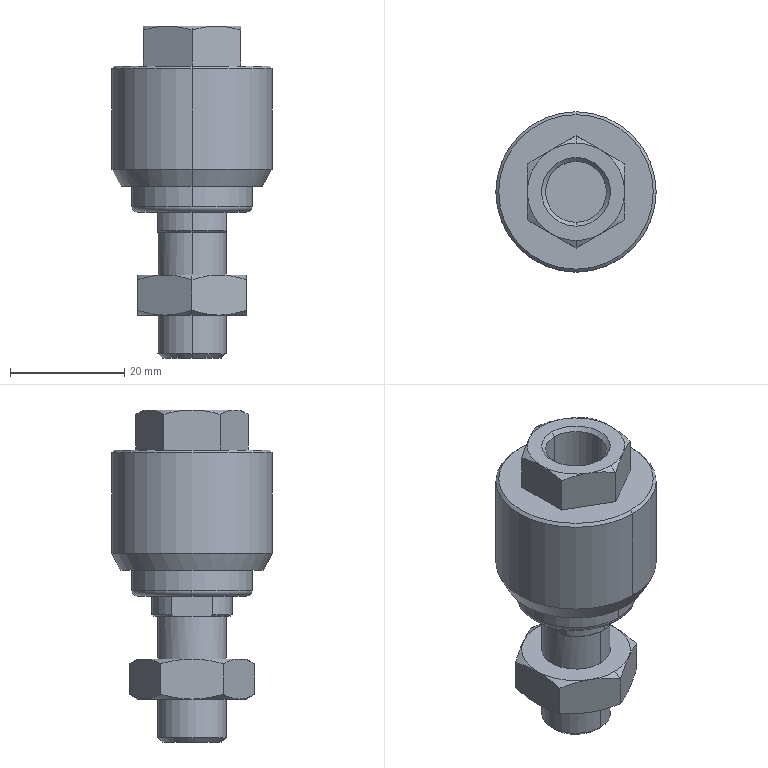Part | SolidWorks | features BaseBody 1 | 1 solid | 91 faces | box 28 x 28 x 58 mm | volume 19286 mm3 | cone 45 | plane 25 | cylinder 19 | torus 2 | commonest cylinder face diameters 12 x6 14 x4 10.647 x3 21 x3 28 x3